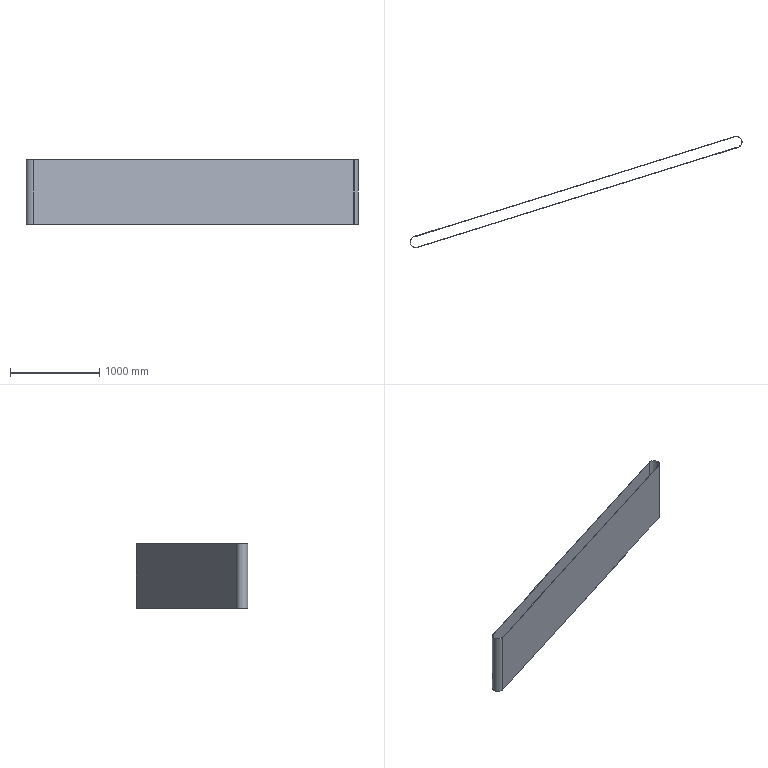Part | SolidWorks | features Extrusion 1 | 1 solid | 12 faces | box 3723 x 1248 x 720 mm | volume 17109923 mm3 | cylinder 6 | plane 6 | commonest cylinder face diameters 120 x3 126 x3
STEP:
#1=CARTESIAN_POINT('',(3392.633,1766.778,-360.));
#2=VERTEX_POINT('',#1);
#3=CARTESIAN_POINT('',(3470.5,1709.5,-360.));
#4=VERTEX_POINT('',#3);
#5=CARTESIAN_POINT('',(3410.5,1709.5,-360.));
#6=DIRECTION('',(0.,0.,-1.));
#7=DIRECTION('',(0.,-1.,0.));
#8=AXIS2_PLACEMENT_3D('',#5,#6,#7);
#9=CIRCLE('',#8,60.);
#10=EDGE_CURVE('',#2,#4,#9,.T.);
#11=ORIENTED_EDGE('',*,*,#10,.T.);
#12=CARTESIAN_POINT('',(3470.5,1709.5,360.));
#13=VERTEX_POINT('',#12);
#14=CARTESIAN_POINT('',(3470.5,1709.5,-4286.1));
#15=DIRECTION('',(0.,0.,1.));
#16=VECTOR('',#15,1000.);
#17=LINE('',#14,#16);
#18=EDGE_CURVE('',#4,#13,#17,.T.);
#19=ORIENTED_EDGE('',*,*,#18,.T.);
#20=CARTESIAN_POINT('',(3392.633,1766.778,360.));
#21=VERTEX_POINT('',#20);
#22=CARTESIAN_POINT('',(3410.5,1709.5,360.));
#23=DIRECTION('',(0.,0.,1.));
#24=DIRECTION('',(1.,0.,0.));
#25=AXIS2_PLACEMENT_3D('',#22,#23,#24);
#26=CIRCLE('',#25,60.);
#27=EDGE_CURVE('',#13,#21,#26,.T.);
#28=ORIENTED_EDGE('',*,*,#27,.T.);
#29=CARTESIAN_POINT('',(3392.633,1766.778,-4286.1));
#30=DIRECTION('',(0.,0.,1.));
#31=VECTOR('',#30,1000.);
#32=LINE('',#29,#31);
#33=EDGE_CURVE('',#2,#21,#32,.T.);
#34=ORIENTED_EDGE('',*,*,#33,.F.);
#35=EDGE_LOOP('',(#11,#19,#28,#34));
#36=FACE_OUTER_BOUND('',#35,.T.);
#37=CARTESIAN_POINT('',(3410.5,1709.5,-4286.1));
#38=DIRECTION('',(0.,0.,1.));
#39=DIRECTION('',(1.,0.,0.));
#40=AXIS2_PLACEMENT_3D('',#37,#38,#39);
#41=CYLINDRICAL_SURFACE('',#40,60.);
#42=ADVANCED_FACE('',(#36),#41,.F.);
#43=CARTESIAN_POINT('',(3473.5,1709.5,-360.));
#44=VERTEX_POINT('',#43);
#45=CARTESIAN_POINT('',(3429.261,1649.358,-360.));
#46=VERTEX_POINT('',#45);
#47=CARTESIAN_POINT('',(3410.5,1709.5,-360.));
#48=DIRECTION('',(0.,0.,-1.));
#49=DIRECTION('',(0.,-1.,0.));
#50=AXIS2_PLACEMENT_3D('',#47,#48,#49);
#51=CIRCLE('',#50,63.);
#52=EDGE_CURVE('',#44,#46,#51,.T.);
#53=ORIENTED_EDGE('',*,*,#52,.F.);
#54=CARTESIAN_POINT('',(3473.5,1709.5,360.));
#55=VERTEX_POINT('',#54);
#56=CARTESIAN_POINT('',(3473.5,1709.5,-4286.1));
#57=DIRECTION('',(0.,0.,1.));
#58=VECTOR('',#57,1000.);
#59=LINE('',#56,#58);
#60=EDGE_CURVE('',#44,#55,#59,.T.);
#61=ORIENTED_EDGE('',*,*,#60,.T.);
#62=CARTESIAN_POINT('',(3429.261,1649.358,360.));
#63=VERTEX_POINT('',#62);
#64=CARTESIAN_POINT('',(3410.5,1709.5,360.));
#65=DIRECTION('',(0.,0.,1.));
#66=DIRECTION('',(1.,0.,0.));
#67=AXIS2_PLACEMENT_3D('',#64,#65,#66);
#68=CIRCLE('',#67,63.);
#69=EDGE_CURVE('',#63,#55,#68,.T.);
#70=ORIENTED_EDGE('',*,*,#69,.F.);
#71=CARTESIAN_POINT('',(3429.261,1649.358,-4286.1));
#72=DIRECTION('',(0.,0.,1.));
#73=VECTOR('',#72,1000.);
#74=LINE('',#71,#73);
#75=EDGE_CURVE('',#46,#63,#74,.T.);
#76=ORIENTED_EDGE('',*,*,#75,.F.);
#77=EDGE_LOOP('',(#53,#61,#70,#76));
#78=FACE_OUTER_BOUND('',#77,.T.);
#79=CARTESIAN_POINT('',(3410.5,1709.5,-4286.1));
#80=DIRECTION('',(0.,0.,1.));
#81=DIRECTION('',(1.,0.,0.));
#82=AXIS2_PLACEMENT_3D('',#79,#80,#81);
#83=CYLINDRICAL_SURFACE('',#82,63.);
#84=ADVANCED_FACE('',(#78),#83,.T.);
#85=CARTESIAN_POINT('',(-167.239,527.458,-360.));
#86=VERTEX_POINT('',#85);
#87=CARTESIAN_POINT('',(-167.239,527.458,-360.));
#88=DIRECTION('',(-0.9546,-0.2978,0.));
#89=VECTOR('',#88,1000.);
#90=LINE('',#87,#89);
#91=EDGE_CURVE('',#46,#86,#90,.T.);
#92=ORIENTED_EDGE('',*,*,#91,.F.);
#93=ORIENTED_EDGE('',*,*,#75,.T.);
#94=CARTESIAN_POINT('',(-167.239,527.458,360.));
#95=VERTEX_POINT('',#94);
#96=CARTESIAN_POINT('',(-167.239,527.458,360.));
#97=DIRECTION('',(0.9546,0.2978,0.));
#98=VECTOR('',#97,1000.);
#99=LINE('',#96,#98);
#100=EDGE_CURVE('',#95,#63,#99,.T.);
#101=ORIENTED_EDGE('',*,*,#100,.F.);
#102=CARTESIAN_POINT('',(-167.239,527.458,-4286.1));
#103=DIRECTION('',(0.,0.,1.));
#104=VECTOR('',#103,1000.);
#105=LINE('',#102,#104);
#106=EDGE_CURVE('',#86,#95,#105,.T.);
#107=ORIENTED_EDGE('',*,*,#106,.F.);
#108=EDGE_LOOP('',(#92,#93,#101,#107));
#109=FACE_OUTER_BOUND('',#108,.T.);
#110=CARTESIAN_POINT('',(-167.239,527.458,-4286.1));
#111=DIRECTION('',(0.2978,-0.9546,0.));
#112=DIRECTION('',(0.9546,0.2978,0.));
#113=AXIS2_PLACEMENT_3D('',#110,#111,#112);
#114=PLANE('',#113);
#115=ADVANCED_FACE('',(#109),#114,.T.);
#116=ORIENTED_EDGE('',*,*,#60,.F.);
#117=CARTESIAN_POINT('',(3391.739,1769.642,-360.));
#118=VERTEX_POINT('',#117);
#119=CARTESIAN_POINT('',(3410.5,1709.5,-360.));
#120=DIRECTION('',(0.,0.,-1.));
#121=DIRECTION('',(0.,-1.,0.));
#122=AXIS2_PLACEMENT_3D('',#119,#120,#121);
#123=CIRCLE('',#122,63.);
#124=EDGE_CURVE('',#118,#44,#123,.T.);
#125=ORIENTED_EDGE('',*,*,#124,.F.);
#126=CARTESIAN_POINT('',(3391.739,1769.642,360.));
#127=VERTEX_POINT('',#126);
#128=CARTESIAN_POINT('',(3391.739,1769.642,-4286.1));
#129=DIRECTION('',(0.,0.,1.));
#130=VECTOR('',#129,1000.);
#131=LINE('',#128,#130);
#132=EDGE_CURVE('',#118,#127,#131,.T.);
#133=ORIENTED_EDGE('',*,*,#132,.T.);
#134=CARTESIAN_POINT('',(3410.5,1709.5,360.));
#135=DIRECTION('',(0.,0.,1.));
#136=DIRECTION('',(1.,0.,0.));
#137=AXIS2_PLACEMENT_3D('',#134,#135,#136);
#138=CIRCLE('',#137,63.);
#139=EDGE_CURVE('',#55,#127,#138,.T.);
#140=ORIENTED_EDGE('',*,*,#139,.F.);
#141=EDGE_LOOP('',(#116,#125,#133,#140));
#142=FACE_OUTER_BOUND('',#141,.T.);
#143=CARTESIAN_POINT('',(3410.5,1709.5,-4286.1));
#144=DIRECTION('',(0.,0.,1.));
#145=DIRECTION('',(1.,0.,0.));
#146=AXIS2_PLACEMENT_3D('',#143,#144,#145);
#147=CYLINDRICAL_SURFACE('',#146,63.);
#148=ADVANCED_FACE('',(#142),#147,.T.);
#149=CARTESIAN_POINT('',(-204.761,647.742,-360.));
#150=VERTEX_POINT('',#149);
#151=CARTESIAN_POINT('',(-204.761,647.742,-360.));
#152=DIRECTION('',(0.9546,0.2978,0.));
#153=VECTOR('',#152,1000.);
#154=LINE('',#151,#153);
#155=EDGE_CURVE('',#150,#118,#154,.T.);
#156=ORIENTED_EDGE('',*,*,#155,.F.);
#157=CARTESIAN_POINT('',(-204.761,647.742,360.));
#158=VERTEX_POINT('',#157);
#159=CARTESIAN_POINT('',(-204.761,647.742,-4286.1));
#160=DIRECTION('',(0.,0.,1.));
#161=VECTOR('',#160,1000.);
#162=LINE('',#159,#161);
#163=EDGE_CURVE('',#150,#158,#162,.T.);
#164=ORIENTED_EDGE('',*,*,#163,.T.);
#165=CARTESIAN_POINT('',(-204.761,647.742,360.));
#166=DIRECTION('',(-0.9546,-0.2978,0.));
#167=VECTOR('',#166,1000.);
#168=LINE('',#165,#167);
#169=EDGE_CURVE('',#127,#158,#168,.T.);
#170=ORIENTED_EDGE('',*,*,#169,.F.);
#171=ORIENTED_EDGE('',*,*,#132,.F.);
#172=EDGE_LOOP('',(#156,#164,#170,#171));
#173=FACE_OUTER_BOUND('',#172,.T.);
#174=CARTESIAN_POINT('',(-204.761,647.742,-4286.1));
#175=DIRECTION('',(-0.2978,0.9546,0.));
#176=DIRECTION('',(-0.9546,-0.2978,0.));
#177=AXIS2_PLACEMENT_3D('',#174,#175,#176);
#178=PLANE('',#177);
#179=ADVANCED_FACE('',(#173),#178,.T.);
#180=CARTESIAN_POINT('',(-186.,587.6,-360.));
#181=DIRECTION('',(0.,0.,-1.));
#182=DIRECTION('',(0.,-1.,0.));
#183=AXIS2_PLACEMENT_3D('',#180,#181,#182);
#184=CIRCLE('',#183,63.);
#185=EDGE_CURVE('',#86,#150,#184,.T.);
#186=ORIENTED_EDGE('',*,*,#185,.F.);
#187=ORIENTED_EDGE('',*,*,#106,.T.);
#188=CARTESIAN_POINT('',(-186.,587.6,360.));
#189=DIRECTION('',(0.,0.,1.));
#190=DIRECTION('',(1.,0.,0.));
#191=AXIS2_PLACEMENT_3D('',#188,#189,#190);
#192=CIRCLE('',#191,63.);
#193=EDGE_CURVE('',#158,#95,#192,.T.);
#194=ORIENTED_EDGE('',*,*,#193,.F.);
#195=ORIENTED_EDGE('',*,*,#163,.F.);
#196=EDGE_LOOP('',(#186,#187,#194,#195));
#197=FACE_OUTER_BOUND('',#196,.T.);
#198=CARTESIAN_POINT('',(-186.,587.6,-4286.1));
#199=DIRECTION('',(0.,0.,1.));
#200=DIRECTION('',(1.,0.,0.));
#201=AXIS2_PLACEMENT_3D('',#198,#199,#200);
#202=CYLINDRICAL_SURFACE('',#201,63.);
#203=ADVANCED_FACE('',(#197),#202,.T.);
#204=CARTESIAN_POINT('',(-203.867,644.878,360.));
#205=VERTEX_POINT('',#204);
#206=CARTESIAN_POINT('',(-168.133,530.322,360.));
#207=VERTEX_POINT('',#206);
#208=CARTESIAN_POINT('',(-186.,587.6,360.));
#209=DIRECTION('',(0.,0.,1.));
#210=DIRECTION('',(1.,0.,0.));
#211=AXIS2_PLACEMENT_3D('',#208,#209,#210);
#212=CIRCLE('',#211,60.);
#213=EDGE_CURVE('',#205,#207,#212,.T.);
#214=ORIENTED_EDGE('',*,*,#213,.F.);
#215=CARTESIAN_POINT('',(-203.867,644.878,360.));
#216=DIRECTION('',(-0.9546,-0.2978,0.));
#217=VECTOR('',#216,1000.);
#218=LINE('',#215,#217);
#219=EDGE_CURVE('',#21,#205,#218,.T.);
#220=ORIENTED_EDGE('',*,*,#219,.F.);
#221=ORIENTED_EDGE('',*,*,#27,.F.);
#222=CARTESIAN_POINT('',(3428.367,1652.222,360.));
#223=VERTEX_POINT('',#222);
#224=CARTESIAN_POINT('',(3410.5,1709.5,360.));
#225=DIRECTION('',(0.,0.,1.));
#226=DIRECTION('',(1.,0.,0.));
#227=AXIS2_PLACEMENT_3D('',#224,#225,#226);
#228=CIRCLE('',#227,60.);
#229=EDGE_CURVE('',#223,#13,#228,.T.);
#230=ORIENTED_EDGE('',*,*,#229,.F.);
#231=CARTESIAN_POINT('',(-168.133,530.322,360.));
#232=DIRECTION('',(0.9546,0.2978,0.));
#233=VECTOR('',#232,1000.);
#234=LINE('',#231,#233);
#235=EDGE_CURVE('',#207,#223,#234,.T.);
#236=ORIENTED_EDGE('',*,*,#235,.F.);
#237=EDGE_LOOP('',(#214,#220,#221,#230,#236));
#238=FACE_BOUND('',#237,.T.);
#239=ORIENTED_EDGE('',*,*,#193,.T.);
#240=ORIENTED_EDGE('',*,*,#100,.T.);
#241=ORIENTED_EDGE('',*,*,#69,.T.);
#242=ORIENTED_EDGE('',*,*,#139,.T.);
#243=ORIENTED_EDGE('',*,*,#169,.T.);
#244=EDGE_LOOP('',(#239,#240,#241,#242,#243));
#245=FACE_OUTER_BOUND('',#244,.T.);
#246=CARTESIAN_POINT('',(-186.,587.6,360.));
#247=DIRECTION('',(0.,0.,1.));
#248=DIRECTION('',(1.,0.,0.));
#249=AXIS2_PLACEMENT_3D('',#246,#247,#248);
#250=PLANE('',#249);
#251=ADVANCED_FACE('',(#238,#245),#250,.T.);
#252=CARTESIAN_POINT('',(3428.367,1652.222,-360.));
#253=VERTEX_POINT('',#252);
#254=CARTESIAN_POINT('',(3428.367,1652.222,-4286.1));
#255=DIRECTION('',(0.,0.,1.));
#256=VECTOR('',#255,1000.);
#257=LINE('',#254,#256);
#258=EDGE_CURVE('',#253,#223,#257,.T.);
#259=ORIENTED_EDGE('',*,*,#258,.F.);
#260=CARTESIAN_POINT('',(-168.133,530.322,-360.));
#261=VERTEX_POINT('',#260);
#262=CARTESIAN_POINT('',(-168.133,530.322,-360.));
#263=DIRECTION('',(-0.9546,-0.2978,0.));
#264=VECTOR('',#263,1000.);
#265=LINE('',#262,#264);
#266=EDGE_CURVE('',#253,#261,#265,.T.);
#267=ORIENTED_EDGE('',*,*,#266,.T.);
#268=CARTESIAN_POINT('',(-168.133,530.322,-4286.1));
#269=DIRECTION('',(0.,0.,1.));
#270=VECTOR('',#269,1000.);
#271=LINE('',#268,#270);
#272=EDGE_CURVE('',#261,#207,#271,.T.);
#273=ORIENTED_EDGE('',*,*,#272,.T.);
#274=ORIENTED_EDGE('',*,*,#235,.T.);
#275=EDGE_LOOP('',(#259,#267,#273,#274));
#276=FACE_OUTER_BOUND('',#275,.T.);
#277=CARTESIAN_POINT('',(-168.133,530.322,-4286.1));
#278=DIRECTION('',(0.2978,-0.9546,0.));
#279=DIRECTION('',(0.9546,0.2978,0.));
#280=AXIS2_PLACEMENT_3D('',#277,#278,#279);
#281=PLANE('',#280);
#282=ADVANCED_FACE('',(#276),#281,.F.);
#283=ORIENTED_EDGE('',*,*,#18,.F.);
#284=CARTESIAN_POINT('',(3410.5,1709.5,-360.));
#285=DIRECTION('',(0.,0.,-1.));
#286=DIRECTION('',(0.,-1.,0.));
#287=AXIS2_PLACEMENT_3D('',#284,#285,#286);
#288=CIRCLE('',#287,60.);
#289=EDGE_CURVE('',#4,#253,#288,.T.);
#290=ORIENTED_EDGE('',*,*,#289,.T.);
#291=ORIENTED_EDGE('',*,*,#258,.T.);
#292=ORIENTED_EDGE('',*,*,#229,.T.);
#293=EDGE_LOOP('',(#283,#290,#291,#292));
#294=FACE_OUTER_BOUND('',#293,.T.);
#295=CARTESIAN_POINT('',(3410.5,1709.5,-4286.1));
#296=DIRECTION('',(0.,0.,1.));
#297=DIRECTION('',(1.,0.,0.));
#298=AXIS2_PLACEMENT_3D('',#295,#296,#297);
#299=CYLINDRICAL_SURFACE('',#298,60.);
#300=ADVANCED_FACE('',(#294),#299,.F.);
#301=CARTESIAN_POINT('',(-203.867,644.878,-360.));
#302=VERTEX_POINT('',#301);
#303=CARTESIAN_POINT('',(-203.867,644.878,-4286.1));
#304=DIRECTION('',(0.,0.,1.));
#305=VECTOR('',#304,1000.);
#306=LINE('',#303,#305);
#307=EDGE_CURVE('',#302,#205,#306,.T.);
#308=ORIENTED_EDGE('',*,*,#307,.F.);
#309=CARTESIAN_POINT('',(-203.867,644.878,-360.));
#310=DIRECTION('',(0.9546,0.2978,0.));
#311=VECTOR('',#310,1000.);
#312=LINE('',#309,#311);
#313=EDGE_CURVE('',#302,#2,#312,.T.);
#314=ORIENTED_EDGE('',*,*,#313,.T.);
#315=ORIENTED_EDGE('',*,*,#33,.T.);
#316=ORIENTED_EDGE('',*,*,#219,.T.);
#317=EDGE_LOOP('',(#308,#314,#315,#316));
#318=FACE_OUTER_BOUND('',#317,.T.);
#319=CARTESIAN_POINT('',(-203.867,644.878,-4286.1));
#320=DIRECTION('',(-0.2978,0.9546,0.));
#321=DIRECTION('',(-0.9546,-0.2978,0.));
#322=AXIS2_PLACEMENT_3D('',#319,#320,#321);
#323=PLANE('',#322);
#324=ADVANCED_FACE('',(#318),#323,.F.);
#325=ORIENTED_EDGE('',*,*,#272,.F.);
#326=CARTESIAN_POINT('',(-186.,587.6,-360.));
#327=DIRECTION('',(0.,0.,-1.));
#328=DIRECTION('',(0.,-1.,0.));
#329=AXIS2_PLACEMENT_3D('',#326,#327,#328);
#330=CIRCLE('',#329,60.);
#331=EDGE_CURVE('',#261,#302,#330,.T.);
#332=ORIENTED_EDGE('',*,*,#331,.T.);
#333=ORIENTED_EDGE('',*,*,#307,.T.);
#334=ORIENTED_EDGE('',*,*,#213,.T.);
#335=EDGE_LOOP('',(#325,#332,#333,#334));
#336=FACE_OUTER_BOUND('',#335,.T.);
#337=CARTESIAN_POINT('',(-186.,587.6,-4286.1));
#338=DIRECTION('',(0.,0.,1.));
#339=DIRECTION('',(1.,0.,0.));
#340=AXIS2_PLACEMENT_3D('',#337,#338,#339);
#341=CYLINDRICAL_SURFACE('',#340,60.);
#342=ADVANCED_FACE('',(#336),#341,.F.);
#343=ORIENTED_EDGE('',*,*,#185,.T.);
#344=ORIENTED_EDGE('',*,*,#155,.T.);
#345=ORIENTED_EDGE('',*,*,#124,.T.);
#346=ORIENTED_EDGE('',*,*,#52,.T.);
#347=ORIENTED_EDGE('',*,*,#91,.T.);
#348=EDGE_LOOP('',(#343,#344,#345,#346,#347));
#349=FACE_OUTER_BOUND('',#348,.T.);
#350=ORIENTED_EDGE('',*,*,#266,.F.);
#351=ORIENTED_EDGE('',*,*,#289,.F.);
#352=ORIENTED_EDGE('',*,*,#10,.F.);
#353=ORIENTED_EDGE('',*,*,#313,.F.);
#354=ORIENTED_EDGE('',*,*,#331,.F.);
#355=EDGE_LOOP('',(#350,#351,#352,#353,#354));
#356=FACE_BOUND('',#355,.T.);
#357=CARTESIAN_POINT('',(3410.5,1769.5,-360.));
#358=DIRECTION('',(0.,0.,1.));
#359=DIRECTION('',(0.,-1.,0.));
#360=AXIS2_PLACEMENT_3D('',#357,#358,#359);
#361=PLANE('',#360);
#362=ADVANCED_FACE('',(#349,#356),#361,.F.);
#363=CLOSED_SHELL('',(#42,#84,#115,#148,#179,#203,#251,#282,#300,#324,#342,#362));
#364=MANIFOLD_SOLID_BREP('',#363);
#365=CARTESIAN_POINT('',(0.,0.,0.));
#366=DIRECTION('',(0.,0.,1.));
#367=DIRECTION('',(1.,0.,0.));
#368=AXIS2_PLACEMENT_3D('',#365,#366,#367);
#369=(LENGTH_UNIT()NAMED_UNIT(*)SI_UNIT(.MILLI.,.METRE.));
#370=UNCERTAINTY_MEASURE_WITH_UNIT(LENGTH_MEASURE(0.00001),#369,'','');
#371=(NAMED_UNIT(*)PLANE_ANGLE_UNIT()SI_UNIT($,.RADIAN.));
#372=(NAMED_UNIT(*)SI_UNIT($,.STERADIAN.)SOLID_ANGLE_UNIT());
#373=(GEOMETRIC_REPRESENTATION_CONTEXT(3)GLOBAL_UNCERTAINTY_ASSIGNED_CONTEXT((#370))GLOBAL_UNIT_ASSIGNED_CONTEXT((#369,#371,#372))REPRESENTATION_CONTEXT('',''));
#374=ADVANCED_BREP_SHAPE_REPRESENTATION('',(#364,#368),#373);